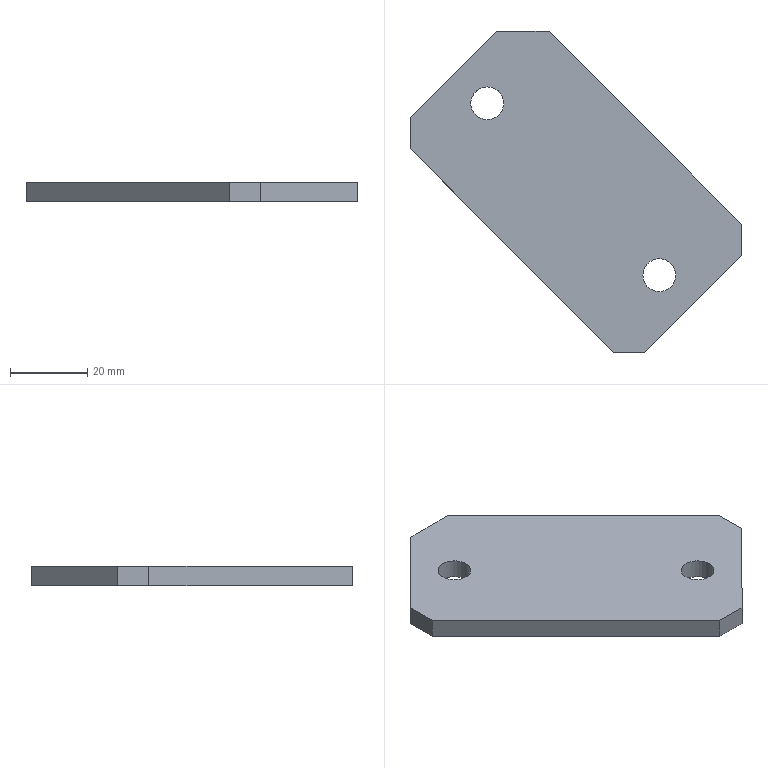Part | STEP file | gslz 2016.10.28-13_id546_x_t | 1 solid | 12 faces | box 85.974 x 83.146 x 5 mm | volume 19163 mm3 | plane 10 | cylinder 2 | commonest cylinder face diameters 8.5 x2
STEP:
#1=CARTESIAN_POINT('',(0.,0.,0.));
#2=DIRECTION('',(0.,0.,1.));
#3=DIRECTION('',(1.,0.,0.));
#4=AXIS2_PLACEMENT_3D('',#1,#2,#3);
#5=CARTESIAN_POINT('',(170.764,264.917,-94.));
#6=VERTEX_POINT('',#5);
#7=CARTESIAN_POINT('',(148.429,242.582,-94.));
#8=VERTEX_POINT('',#7);
#9=CARTESIAN_POINT('',(177.981,272.134,-94.));
#10=DIRECTION('',(-0.7071,-0.7071,0.));
#11=VECTOR('',#10,1.);
#12=LINE('',#9,#11);
#13=CARTESIAN_POINT('',(177.981,272.134,-99.));
#14=DIRECTION('',(-0.7071,0.7071,0.));
#15=DIRECTION('',(-0.7071,-0.7071,0.));
#16=AXIS2_PLACEMENT_3D('',#13,#14,#15);
#17=PLANE('',#16);
#18=CARTESIAN_POINT('',(0.,5.));
#19=DIRECTION('',(1.,0.));
#20=VECTOR('',#19,1.);
#21=LINE('',#18,#20);
#22=(GEOMETRIC_REPRESENTATION_CONTEXT(2)PARAMETRIC_REPRESENTATION_CONTEXT()REPRESENTATION_CONTEXT('',''));
#23=DEFINITIONAL_REPRESENTATION('',(#21),#22);
#24=PCURVE('',#17,#23);
#25=CARTESIAN_POINT('',(-1012.771,1462.886,-94.));
#26=DIRECTION('',(0.,0.,1.));
#27=DIRECTION('',(1.,0.,0.));
#28=AXIS2_PLACEMENT_3D('',#25,#26,#27);
#29=PLANE('',#28);
#30=CARTESIAN_POINT('',(1190.752,-1190.752));
#31=DIRECTION('',(-0.7071,-0.7071));
#32=VECTOR('',#31,1.);
#33=LINE('',#30,#32);
#34=(GEOMETRIC_REPRESENTATION_CONTEXT(2)PARAMETRIC_REPRESENTATION_CONTEXT()REPRESENTATION_CONTEXT('',''));
#35=DEFINITIONAL_REPRESENTATION('',(#33),#34);
#36=PCURVE('',#29,#35);
#37=SURFACE_CURVE('',#12,(#24,#36),.PCURVE_S1.);
#38=EDGE_CURVE('',#6,#8,#37,.T.);
#39=ORIENTED_EDGE('',*,*,#38,.F.);
#40=CARTESIAN_POINT('',(170.764,264.917,-99.));
#41=VERTEX_POINT('',#40);
#42=CARTESIAN_POINT('',(170.764,264.917,-99.));
#43=DIRECTION('',(0.,0.,1.));
#44=VECTOR('',#43,1.);
#45=LINE('',#42,#44);
#46=CARTESIAN_POINT('',(10.207,0.));
#47=DIRECTION('',(0.,1.));
#48=VECTOR('',#47,1.);
#49=LINE('',#46,#48);
#50=(GEOMETRIC_REPRESENTATION_CONTEXT(2)PARAMETRIC_REPRESENTATION_CONTEXT()REPRESENTATION_CONTEXT('',''));
#51=DEFINITIONAL_REPRESENTATION('',(#49),#50);
#52=PCURVE('',#17,#51);
#53=CARTESIAN_POINT('',(184.699,264.917,-99.));
#54=DIRECTION('',(0.,-1.,0.));
#55=DIRECTION('',(1.,0.,0.));
#56=AXIS2_PLACEMENT_3D('',#53,#54,#55);
#57=PLANE('',#56);
#58=CARTESIAN_POINT('',(-13.935,0.));
#59=DIRECTION('',(0.,1.));
#60=VECTOR('',#59,1.);
#61=LINE('',#58,#60);
#62=(GEOMETRIC_REPRESENTATION_CONTEXT(2)PARAMETRIC_REPRESENTATION_CONTEXT()REPRESENTATION_CONTEXT('',''));
#63=DEFINITIONAL_REPRESENTATION('',(#61),#62);
#64=PCURVE('',#57,#63);
#65=SURFACE_CURVE('',#45,(#52,#64),.PCURVE_S1.);
#66=EDGE_CURVE('',#41,#6,#65,.T.);
#67=ORIENTED_EDGE('',*,*,#66,.F.);
#68=CARTESIAN_POINT('',(148.429,242.582,-99.));
#69=VERTEX_POINT('',#68);
#70=CARTESIAN_POINT('',(177.981,272.134,-99.));
#71=DIRECTION('',(-0.7071,-0.7071,0.));
#72=VECTOR('',#71,1.);
#73=LINE('',#70,#72);
#74=CARTESIAN_POINT('',(0.,0.));
#75=DIRECTION('',(1.,0.));
#76=VECTOR('',#75,1.);
#77=LINE('',#74,#76);
#78=(GEOMETRIC_REPRESENTATION_CONTEXT(2)PARAMETRIC_REPRESENTATION_CONTEXT()REPRESENTATION_CONTEXT('',''));
#79=DEFINITIONAL_REPRESENTATION('',(#77),#78);
#80=PCURVE('',#17,#79);
#81=CARTESIAN_POINT('',(-1012.771,1462.886,-99.));
#82=DIRECTION('',(0.,0.,1.));
#83=DIRECTION('',(1.,0.,0.));
#84=AXIS2_PLACEMENT_3D('',#81,#82,#83);
#85=PLANE('',#84);
#86=CARTESIAN_POINT('',(1190.752,-1190.752));
#87=DIRECTION('',(-0.7071,-0.7071));
#88=VECTOR('',#87,1.);
#89=LINE('',#86,#88);
#90=(GEOMETRIC_REPRESENTATION_CONTEXT(2)PARAMETRIC_REPRESENTATION_CONTEXT()REPRESENTATION_CONTEXT('',''));
#91=DEFINITIONAL_REPRESENTATION('',(#89),#90);
#92=PCURVE('',#85,#91);
#93=SURFACE_CURVE('',#73,(#80,#92),.PCURVE_S1.);
#94=EDGE_CURVE('',#41,#69,#93,.T.);
#95=ORIENTED_EDGE('',*,*,#94,.T.);
#96=CARTESIAN_POINT('',(148.429,242.582,-99.));
#97=DIRECTION('',(0.,0.,1.));
#98=VECTOR('',#97,1.);
#99=LINE('',#96,#98);
#100=CARTESIAN_POINT('',(41.793,0.));
#101=DIRECTION('',(0.,1.));
#102=VECTOR('',#101,1.);
#103=LINE('',#100,#102);
#104=(GEOMETRIC_REPRESENTATION_CONTEXT(2)PARAMETRIC_REPRESENTATION_CONTEXT()REPRESENTATION_CONTEXT('',''));
#105=DEFINITIONAL_REPRESENTATION('',(#103),#104);
#106=PCURVE('',#17,#105);
#107=CARTESIAN_POINT('',(148.429,242.789,-99.));
#108=DIRECTION('',(1.,0.,0.));
#109=DIRECTION('',(0.,1.,0.));
#110=AXIS2_PLACEMENT_3D('',#107,#108,#109);
#111=PLANE('',#110);
#112=CARTESIAN_POINT('',(-0.2071,0.));
#113=DIRECTION('',(0.,1.));
#114=VECTOR('',#113,1.);
#115=LINE('',#112,#114);
#116=(GEOMETRIC_REPRESENTATION_CONTEXT(2)PARAMETRIC_REPRESENTATION_CONTEXT()REPRESENTATION_CONTEXT('',''));
#117=DEFINITIONAL_REPRESENTATION('',(#115),#116);
#118=PCURVE('',#111,#117);
#119=SURFACE_CURVE('',#99,(#106,#118),.PCURVE_S1.);
#120=EDGE_CURVE('',#69,#8,#119,.T.);
#121=ORIENTED_EDGE('',*,*,#120,.T.);
#122=EDGE_LOOP('',(#39,#67,#95,#121));
#123=FACE_BOUND('',#122,.T.);
#124=ADVANCED_FACE('',(#123),#17,.T.);
#125=CARTESIAN_POINT('',(184.492,264.917,-94.));
#126=VERTEX_POINT('',#125);
#127=CARTESIAN_POINT('',(-1012.771,264.917,-94.));
#128=DIRECTION('',(1.,0.,0.));
#129=VECTOR('',#128,1.);
#130=LINE('',#127,#129);
#131=CARTESIAN_POINT('',(-1197.469,5.));
#132=DIRECTION('',(1.,0.));
#133=VECTOR('',#132,1.);
#134=LINE('',#131,#133);
#135=(GEOMETRIC_REPRESENTATION_CONTEXT(2)PARAMETRIC_REPRESENTATION_CONTEXT()REPRESENTATION_CONTEXT('',''));
#136=DEFINITIONAL_REPRESENTATION('',(#134),#135);
#137=PCURVE('',#57,#136);
#138=CARTESIAN_POINT('',(0.,-1197.969));
#139=DIRECTION('',(1.,0.));
#140=VECTOR('',#139,1.);
#141=LINE('',#138,#140);
#142=(GEOMETRIC_REPRESENTATION_CONTEXT(2)PARAMETRIC_REPRESENTATION_CONTEXT()REPRESENTATION_CONTEXT('',''));
#143=DEFINITIONAL_REPRESENTATION('',(#141),#142);
#144=PCURVE('',#29,#143);
#145=SURFACE_CURVE('',#130,(#137,#144),.PCURVE_S1.);
#146=EDGE_CURVE('',#6,#126,#145,.T.);
#147=ORIENTED_EDGE('',*,*,#146,.T.);
#148=CARTESIAN_POINT('',(184.492,264.917,-99.));
#149=VERTEX_POINT('',#148);
#150=CARTESIAN_POINT('',(184.492,264.917,-99.));
#151=DIRECTION('',(0.,0.,1.));
#152=VECTOR('',#151,1.);
#153=LINE('',#150,#152);
#154=CARTESIAN_POINT('',(-0.2071,0.));
#155=DIRECTION('',(0.,1.));
#156=VECTOR('',#155,1.);
#157=LINE('',#154,#156);
#158=(GEOMETRIC_REPRESENTATION_CONTEXT(2)PARAMETRIC_REPRESENTATION_CONTEXT()REPRESENTATION_CONTEXT('',''));
#159=DEFINITIONAL_REPRESENTATION('',(#157),#158);
#160=PCURVE('',#57,#159);
#161=CARTESIAN_POINT('',(-1013.124,1462.533,-99.));
#162=DIRECTION('',(0.7071,0.7071,0.));
#163=DIRECTION('',(-0.7071,0.7071,0.));
#164=AXIS2_PLACEMENT_3D('',#161,#162,#163);
#165=PLANE('',#164);
#166=CARTESIAN_POINT('',(-1693.685,0.));
#167=DIRECTION('',(0.,1.));
#168=VECTOR('',#167,1.);
#169=LINE('',#166,#168);
#170=(GEOMETRIC_REPRESENTATION_CONTEXT(2)PARAMETRIC_REPRESENTATION_CONTEXT()REPRESENTATION_CONTEXT('',''));
#171=DEFINITIONAL_REPRESENTATION('',(#169),#170);
#172=PCURVE('',#165,#171);
#173=SURFACE_CURVE('',#153,(#160,#172),.PCURVE_S1.);
#174=EDGE_CURVE('',#149,#126,#173,.T.);
#175=ORIENTED_EDGE('',*,*,#174,.F.);
#176=CARTESIAN_POINT('',(-1012.771,264.917,-99.));
#177=DIRECTION('',(1.,0.,0.));
#178=VECTOR('',#177,1.);
#179=LINE('',#176,#178);
#180=CARTESIAN_POINT('',(-1197.469,0.));
#181=DIRECTION('',(1.,0.));
#182=VECTOR('',#181,1.);
#183=LINE('',#180,#182);
#184=(GEOMETRIC_REPRESENTATION_CONTEXT(2)PARAMETRIC_REPRESENTATION_CONTEXT()REPRESENTATION_CONTEXT('',''));
#185=DEFINITIONAL_REPRESENTATION('',(#183),#184);
#186=PCURVE('',#57,#185);
#187=CARTESIAN_POINT('',(0.,-1197.969));
#188=DIRECTION('',(1.,0.));
#189=VECTOR('',#188,1.);
#190=LINE('',#187,#189);
#191=(GEOMETRIC_REPRESENTATION_CONTEXT(2)PARAMETRIC_REPRESENTATION_CONTEXT()REPRESENTATION_CONTEXT('',''));
#192=DEFINITIONAL_REPRESENTATION('',(#190),#191);
#193=PCURVE('',#85,#192);
#194=SURFACE_CURVE('',#179,(#186,#193),.PCURVE_S1.);
#195=EDGE_CURVE('',#41,#149,#194,.T.);
#196=ORIENTED_EDGE('',*,*,#195,.F.);
#197=ORIENTED_EDGE('',*,*,#66,.T.);
#198=EDGE_LOOP('',(#147,#175,#196,#197));
#199=FACE_BOUND('',#198,.T.);
#200=ADVANCED_FACE('',(#199),#57,.F.);
#201=CARTESIAN_POINT('',(234.403,215.005,-94.));
#202=VERTEX_POINT('',#201);
#203=CARTESIAN_POINT('',(-1013.124,1462.533,-94.));
#204=DIRECTION('',(-0.7071,0.7071,0.));
#205=VECTOR('',#204,1.);
#206=LINE('',#203,#205);
#207=CARTESIAN_POINT('',(0.,5.));
#208=DIRECTION('',(1.,0.));
#209=VECTOR('',#208,1.);
#210=LINE('',#207,#209);
#211=(GEOMETRIC_REPRESENTATION_CONTEXT(2)PARAMETRIC_REPRESENTATION_CONTEXT()REPRESENTATION_CONTEXT('',''));
#212=DEFINITIONAL_REPRESENTATION('',(#210),#211);
#213=PCURVE('',#165,#212);
#214=CARTESIAN_POINT('',(-0.3536,-0.3536));
#215=DIRECTION('',(-0.7071,0.7071));
#216=VECTOR('',#215,1.);
#217=LINE('',#214,#216);
#218=(GEOMETRIC_REPRESENTATION_CONTEXT(2)PARAMETRIC_REPRESENTATION_CONTEXT()REPRESENTATION_CONTEXT('',''));
#219=DEFINITIONAL_REPRESENTATION('',(#217),#218);
#220=PCURVE('',#29,#219);
#221=SURFACE_CURVE('',#206,(#213,#220),.PCURVE_S1.);
#222=EDGE_CURVE('',#202,#126,#221,.T.);
#223=ORIENTED_EDGE('',*,*,#222,.F.);
#224=CARTESIAN_POINT('',(234.403,215.005,-99.));
#225=VERTEX_POINT('',#224);
#226=CARTESIAN_POINT('',(234.403,215.005,-99.));
#227=DIRECTION('',(0.,0.,1.));
#228=VECTOR('',#227,1.);
#229=LINE('',#226,#228);
#230=CARTESIAN_POINT('',(-1764.27,0.));
#231=DIRECTION('',(0.,1.));
#232=VECTOR('',#231,1.);
#233=LINE('',#230,#232);
#234=(GEOMETRIC_REPRESENTATION_CONTEXT(2)PARAMETRIC_REPRESENTATION_CONTEXT()REPRESENTATION_CONTEXT('',''));
#235=DEFINITIONAL_REPRESENTATION('',(#233),#234);
#236=PCURVE('',#165,#235);
#237=CARTESIAN_POINT('',(234.403,206.727,-99.));
#238=DIRECTION('',(-1.,0.,0.));
#239=DIRECTION('',(0.,-1.,0.));
#240=AXIS2_PLACEMENT_3D('',#237,#238,#239);
#241=PLANE('',#240);
#242=CARTESIAN_POINT('',(-8.278,0.));
#243=DIRECTION('',(0.,1.));
#244=VECTOR('',#243,1.);
#245=LINE('',#242,#244);
#246=(GEOMETRIC_REPRESENTATION_CONTEXT(2)PARAMETRIC_REPRESENTATION_CONTEXT()REPRESENTATION_CONTEXT('',''));
#247=DEFINITIONAL_REPRESENTATION('',(#245),#246);
#248=PCURVE('',#241,#247);
#249=SURFACE_CURVE('',#229,(#236,#248),.PCURVE_S1.);
#250=EDGE_CURVE('',#225,#202,#249,.T.);
#251=ORIENTED_EDGE('',*,*,#250,.F.);
#252=CARTESIAN_POINT('',(-1013.124,1462.533,-99.));
#253=DIRECTION('',(-0.7071,0.7071,0.));
#254=VECTOR('',#253,1.);
#255=LINE('',#252,#254);
#256=CARTESIAN_POINT('',(0.,0.));
#257=DIRECTION('',(1.,0.));
#258=VECTOR('',#257,1.);
#259=LINE('',#256,#258);
#260=(GEOMETRIC_REPRESENTATION_CONTEXT(2)PARAMETRIC_REPRESENTATION_CONTEXT()REPRESENTATION_CONTEXT('',''));
#261=DEFINITIONAL_REPRESENTATION('',(#259),#260);
#262=PCURVE('',#165,#261);
#263=CARTESIAN_POINT('',(-0.3536,-0.3536));
#264=DIRECTION('',(-0.7071,0.7071));
#265=VECTOR('',#264,1.);
#266=LINE('',#263,#265);
#267=(GEOMETRIC_REPRESENTATION_CONTEXT(2)PARAMETRIC_REPRESENTATION_CONTEXT()REPRESENTATION_CONTEXT('',''));
#268=DEFINITIONAL_REPRESENTATION('',(#266),#267);
#269=PCURVE('',#85,#268);
#270=SURFACE_CURVE('',#255,(#262,#269),.PCURVE_S1.);
#271=EDGE_CURVE('',#225,#149,#270,.T.);
#272=ORIENTED_EDGE('',*,*,#271,.T.);
#273=ORIENTED_EDGE('',*,*,#174,.T.);
#274=EDGE_LOOP('',(#223,#251,#272,#273));
#275=FACE_BOUND('',#274,.T.);
#276=ADVANCED_FACE('',(#275),#165,.T.);
#277=CARTESIAN_POINT('',(234.403,206.934,-94.));
#278=VERTEX_POINT('',#277);
#279=CARTESIAN_POINT('',(234.403,1462.886,-94.));
#280=DIRECTION('',(0.,-1.,0.));
#281=VECTOR('',#280,1.);
#282=LINE('',#279,#281);
#283=CARTESIAN_POINT('',(-1256.159,5.));
#284=DIRECTION('',(1.,0.));
#285=VECTOR('',#284,1.);
#286=LINE('',#283,#285);
#287=(GEOMETRIC_REPRESENTATION_CONTEXT(2)PARAMETRIC_REPRESENTATION_CONTEXT()REPRESENTATION_CONTEXT('',''));
#288=DEFINITIONAL_REPRESENTATION('',(#286),#287);
#289=PCURVE('',#241,#288);
#290=CARTESIAN_POINT('',(1247.174,0.));
#291=DIRECTION('',(0.,-1.));
#292=VECTOR('',#291,1.);
#293=LINE('',#290,#292);
#294=(GEOMETRIC_REPRESENTATION_CONTEXT(2)PARAMETRIC_REPRESENTATION_CONTEXT()REPRESENTATION_CONTEXT('',''));
#295=DEFINITIONAL_REPRESENTATION('',(#293),#294);
#296=PCURVE('',#29,#295);
#297=SURFACE_CURVE('',#282,(#289,#296),.PCURVE_S1.);
#298=EDGE_CURVE('',#202,#278,#297,.T.);
#299=ORIENTED_EDGE('',*,*,#298,.T.);
#300=CARTESIAN_POINT('',(234.403,206.934,-99.));
#301=VERTEX_POINT('',#300);
#302=CARTESIAN_POINT('',(234.403,206.934,-99.));
#303=DIRECTION('',(0.,0.,1.));
#304=VECTOR('',#303,1.);
#305=LINE('',#302,#304);
#306=CARTESIAN_POINT('',(-0.2071,0.));
#307=DIRECTION('',(0.,1.));
#308=VECTOR('',#307,1.);
#309=LINE('',#306,#308);
#310=(GEOMETRIC_REPRESENTATION_CONTEXT(2)PARAMETRIC_REPRESENTATION_CONTEXT()REPRESENTATION_CONTEXT('',''));
#311=DEFINITIONAL_REPRESENTATION('',(#309),#310);
#312=PCURVE('',#241,#311);
#313=CARTESIAN_POINT('',(238.793,211.323,-99.));
#314=DIRECTION('',(-0.7071,0.7071,0.));
#315=DIRECTION('',(-0.7071,-0.7071,0.));
#316=AXIS2_PLACEMENT_3D('',#313,#314,#315);
#317=PLANE('',#316);
#318=CARTESIAN_POINT('',(6.207,0.));
#319=DIRECTION('',(0.,1.));
#320=VECTOR('',#319,1.);
#321=LINE('',#318,#320);
#322=(GEOMETRIC_REPRESENTATION_CONTEXT(2)PARAMETRIC_REPRESENTATION_CONTEXT()REPRESENTATION_CONTEXT('',''));
#323=DEFINITIONAL_REPRESENTATION('',(#321),#322);
#324=PCURVE('',#317,#323);
#325=SURFACE_CURVE('',#305,(#312,#324),.PCURVE_S1.);
#326=EDGE_CURVE('',#301,#278,#325,.T.);
#327=ORIENTED_EDGE('',*,*,#326,.F.);
#328=CARTESIAN_POINT('',(234.403,1462.886,-99.));
#329=DIRECTION('',(0.,-1.,0.));
#330=VECTOR('',#329,1.);
#331=LINE('',#328,#330);
#332=CARTESIAN_POINT('',(-1256.159,0.));
#333=DIRECTION('',(1.,0.));
#334=VECTOR('',#333,1.);
#335=LINE('',#332,#334);
#336=(GEOMETRIC_REPRESENTATION_CONTEXT(2)PARAMETRIC_REPRESENTATION_CONTEXT()REPRESENTATION_CONTEXT('',''));
#337=DEFINITIONAL_REPRESENTATION('',(#335),#336);
#338=PCURVE('',#241,#337);
#339=CARTESIAN_POINT('',(1247.174,0.));
#340=DIRECTION('',(0.,-1.));
#341=VECTOR('',#340,1.);
#342=LINE('',#339,#341);
#343=(GEOMETRIC_REPRESENTATION_CONTEXT(2)PARAMETRIC_REPRESENTATION_CONTEXT()REPRESENTATION_CONTEXT('',''));
#344=DEFINITIONAL_REPRESENTATION('',(#342),#343);
#345=PCURVE('',#85,#344);
#346=SURFACE_CURVE('',#331,(#338,#345),.PCURVE_S1.);
#347=EDGE_CURVE('',#225,#301,#346,.T.);
#348=ORIENTED_EDGE('',*,*,#347,.F.);
#349=ORIENTED_EDGE('',*,*,#250,.T.);
#350=EDGE_LOOP('',(#299,#327,#348,#349));
#351=FACE_BOUND('',#350,.T.);
#352=ADVANCED_FACE('',(#351),#241,.F.);
#353=CARTESIAN_POINT('',(209.241,181.771,-94.));
#354=VERTEX_POINT('',#353);
#355=CARTESIAN_POINT('',(238.793,211.323,-94.));
#356=DIRECTION('',(-0.7071,-0.7071,0.));
#357=VECTOR('',#356,1.);
#358=LINE('',#355,#357);
#359=CARTESIAN_POINT('',(0.,5.));
#360=DIRECTION('',(1.,0.));
#361=VECTOR('',#360,1.);
#362=LINE('',#359,#361);
#363=(GEOMETRIC_REPRESENTATION_CONTEXT(2)PARAMETRIC_REPRESENTATION_CONTEXT()REPRESENTATION_CONTEXT('',''));
#364=DEFINITIONAL_REPRESENTATION('',(#362),#363);
#365=PCURVE('',#317,#364);
#366=CARTESIAN_POINT('',(1251.563,-1251.563));
#367=DIRECTION('',(-0.7071,-0.7071));
#368=VECTOR('',#367,1.);
#369=LINE('',#366,#368);
#370=(GEOMETRIC_REPRESENTATION_CONTEXT(2)PARAMETRIC_REPRESENTATION_CONTEXT()REPRESENTATION_CONTEXT('',''));
#371=DEFINITIONAL_REPRESENTATION('',(#369),#370);
#372=PCURVE('',#29,#371);
#373=SURFACE_CURVE('',#358,(#365,#372),.PCURVE_S1.);
#374=EDGE_CURVE('',#278,#354,#373,.T.);
#375=ORIENTED_EDGE('',*,*,#374,.T.);
#376=CARTESIAN_POINT('',(209.241,181.771,-99.));
#377=VERTEX_POINT('',#376);
#378=CARTESIAN_POINT('',(209.241,181.771,-99.));
#379=DIRECTION('',(0.,0.,1.));
#380=VECTOR('',#379,1.);
#381=LINE('',#378,#380);
#382=CARTESIAN_POINT('',(41.793,0.));
#383=DIRECTION('',(0.,1.));
#384=VECTOR('',#383,1.);
#385=LINE('',#382,#384);
#386=(GEOMETRIC_REPRESENTATION_CONTEXT(2)PARAMETRIC_REPRESENTATION_CONTEXT()REPRESENTATION_CONTEXT('',''));
#387=DEFINITIONAL_REPRESENTATION('',(#385),#386);
#388=PCURVE('',#317,#387);
#389=CARTESIAN_POINT('',(200.962,181.771,-99.));
#390=DIRECTION('',(0.,1.,0.));
#391=DIRECTION('',(-1.,0.,0.));
#392=AXIS2_PLACEMENT_3D('',#389,#390,#391);
#393=PLANE('',#392);
#394=CARTESIAN_POINT('',(-8.278,0.));
#395=DIRECTION('',(0.,1.));
#396=VECTOR('',#395,1.);
#397=LINE('',#394,#396);
#398=(GEOMETRIC_REPRESENTATION_CONTEXT(2)PARAMETRIC_REPRESENTATION_CONTEXT()REPRESENTATION_CONTEXT('',''));
#399=DEFINITIONAL_REPRESENTATION('',(#397),#398);
#400=PCURVE('',#393,#399);
#401=SURFACE_CURVE('',#381,(#388,#400),.PCURVE_S1.);
#402=EDGE_CURVE('',#377,#354,#401,.T.);
#403=ORIENTED_EDGE('',*,*,#402,.F.);
#404=CARTESIAN_POINT('',(238.793,211.323,-99.));
#405=DIRECTION('',(-0.7071,-0.7071,0.));
#406=VECTOR('',#405,1.);
#407=LINE('',#404,#406);
#408=CARTESIAN_POINT('',(0.,0.));
#409=DIRECTION('',(1.,0.));
#410=VECTOR('',#409,1.);
#411=LINE('',#408,#410);
#412=(GEOMETRIC_REPRESENTATION_CONTEXT(2)PARAMETRIC_REPRESENTATION_CONTEXT()REPRESENTATION_CONTEXT('',''));
#413=DEFINITIONAL_REPRESENTATION('',(#411),#412);
#414=PCURVE('',#317,#413);
#415=CARTESIAN_POINT('',(1251.563,-1251.563));
#416=DIRECTION('',(-0.7071,-0.7071));
#417=VECTOR('',#416,1.);
#418=LINE('',#415,#417);
#419=(GEOMETRIC_REPRESENTATION_CONTEXT(2)PARAMETRIC_REPRESENTATION_CONTEXT()REPRESENTATION_CONTEXT('',''));
#420=DEFINITIONAL_REPRESENTATION('',(#418),#419);
#421=PCURVE('',#85,#420);
#422=SURFACE_CURVE('',#407,(#414,#421),.PCURVE_S1.);
#423=EDGE_CURVE('',#301,#377,#422,.T.);
#424=ORIENTED_EDGE('',*,*,#423,.F.);
#425=ORIENTED_EDGE('',*,*,#326,.T.);
#426=EDGE_LOOP('',(#375,#403,#424,#425));
#427=FACE_BOUND('',#426,.T.);
#428=ADVANCED_FACE('',(#427),#317,.F.);
#429=CARTESIAN_POINT('',(201.169,181.771,-94.));
#430=VERTEX_POINT('',#429);
#431=CARTESIAN_POINT('',(-1012.771,181.771,-94.));
#432=DIRECTION('',(-1.,0.,0.));
#433=VECTOR('',#432,1.);
#434=LINE('',#431,#433);
#435=CARTESIAN_POINT('',(1213.733,5.));
#436=DIRECTION('',(1.,0.));
#437=VECTOR('',#436,1.);
#438=LINE('',#435,#437);
#439=(GEOMETRIC_REPRESENTATION_CONTEXT(2)PARAMETRIC_REPRESENTATION_CONTEXT()REPRESENTATION_CONTEXT('',''));
#440=DEFINITIONAL_REPRESENTATION('',(#438),#439);
#441=PCURVE('',#393,#440);
#442=CARTESIAN_POINT('',(0.,-1281.115));
#443=DIRECTION('',(-1.,0.));
#444=VECTOR('',#443,1.);
#445=LINE('',#442,#444);
#446=(GEOMETRIC_REPRESENTATION_CONTEXT(2)PARAMETRIC_REPRESENTATION_CONTEXT()REPRESENTATION_CONTEXT('',''));
#447=DEFINITIONAL_REPRESENTATION('',(#445),#446);
#448=PCURVE('',#29,#447);
#449=SURFACE_CURVE('',#434,(#441,#448),.PCURVE_S1.);
#450=EDGE_CURVE('',#354,#430,#449,.T.);
#451=ORIENTED_EDGE('',*,*,#450,.T.);
#452=CARTESIAN_POINT('',(201.169,181.771,-99.));
#453=VERTEX_POINT('',#452);
#454=CARTESIAN_POINT('',(201.169,181.771,-99.));
#455=DIRECTION('',(0.,0.,1.));
#456=VECTOR('',#455,1.);
#457=LINE('',#454,#456);
#458=CARTESIAN_POINT('',(-0.2071,0.));
#459=DIRECTION('',(0.,1.));
#460=VECTOR('',#459,1.);
#461=LINE('',#458,#460);
#462=(GEOMETRIC_REPRESENTATION_CONTEXT(2)PARAMETRIC_REPRESENTATION_CONTEXT()REPRESENTATION_CONTEXT('',''));
#463=DEFINITIONAL_REPRESENTATION('',(#461),#462);
#464=PCURVE('',#393,#463);
#465=CARTESIAN_POINT('',(-1046.358,1429.299,-99.));
#466=DIRECTION('',(0.7071,0.7071,0.));
#467=DIRECTION('',(-0.7071,0.7071,0.));
#468=AXIS2_PLACEMENT_3D('',#465,#466,#467);
#469=PLANE('',#468);
#470=CARTESIAN_POINT('',(-1764.27,0.));
#471=DIRECTION('',(0.,1.));
#472=VECTOR('',#471,1.);
#473=LINE('',#470,#472);
#474=(GEOMETRIC_REPRESENTATION_CONTEXT(2)PARAMETRIC_REPRESENTATION_CONTEXT()REPRESENTATION_CONTEXT('',''));
#475=DEFINITIONAL_REPRESENTATION('',(#473),#474);
#476=PCURVE('',#469,#475);
#477=SURFACE_CURVE('',#457,(#464,#476),.PCURVE_S1.);
#478=EDGE_CURVE('',#453,#430,#477,.T.);
#479=ORIENTED_EDGE('',*,*,#478,.F.);
#480=CARTESIAN_POINT('',(-1012.771,181.771,-99.));
#481=DIRECTION('',(-1.,0.,0.));
#482=VECTOR('',#481,1.);
#483=LINE('',#480,#482);
#484=CARTESIAN_POINT('',(1213.733,0.));
#485=DIRECTION('',(1.,0.));
#486=VECTOR('',#485,1.);
#487=LINE('',#484,#486);
#488=(GEOMETRIC_REPRESENTATION_CONTEXT(2)PARAMETRIC_REPRESENTATION_CONTEXT()REPRESENTATION_CONTEXT('',''));
#489=DEFINITIONAL_REPRESENTATION('',(#487),#488);
#490=PCURVE('',#393,#489);
#491=CARTESIAN_POINT('',(0.,-1281.115));
#492=DIRECTION('',(-1.,0.));
#493=VECTOR('',#492,1.);
#494=LINE('',#491,#493);
#495=(GEOMETRIC_REPRESENTATION_CONTEXT(2)PARAMETRIC_REPRESENTATION_CONTEXT()REPRESENTATION_CONTEXT('',''));
#496=DEFINITIONAL_REPRESENTATION('',(#494),#495);
#497=PCURVE('',#85,#496);
#498=SURFACE_CURVE('',#483,(#490,#497),.PCURVE_S1.);
#499=EDGE_CURVE('',#377,#453,#498,.T.);
#500=ORIENTED_EDGE('',*,*,#499,.F.);
#501=ORIENTED_EDGE('',*,*,#402,.T.);
#502=EDGE_LOOP('',(#451,#479,#500,#501));
#503=FACE_BOUND('',#502,.T.);
#504=ADVANCED_FACE('',(#503),#393,.F.);
#505=CARTESIAN_POINT('',(148.429,234.511,-94.));
#506=VERTEX_POINT('',#505);
#507=CARTESIAN_POINT('',(-1046.358,1429.299,-94.));
#508=DIRECTION('',(-0.7071,0.7071,0.));
#509=VECTOR('',#508,1.);
#510=LINE('',#507,#509);
#511=CARTESIAN_POINT('',(0.,5.));
#512=DIRECTION('',(1.,0.));
#513=VECTOR('',#512,1.);
#514=LINE('',#511,#513);
#515=(GEOMETRIC_REPRESENTATION_CONTEXT(2)PARAMETRIC_REPRESENTATION_CONTEXT()REPRESENTATION_CONTEXT('',''));
#516=DEFINITIONAL_REPRESENTATION('',(#514),#515);
#517=PCURVE('',#469,#516);
#518=CARTESIAN_POINT('',(-33.588,-33.588));
#519=DIRECTION('',(-0.7071,0.7071));
#520=VECTOR('',#519,1.);
#521=LINE('',#518,#520);
#522=(GEOMETRIC_REPRESENTATION_CONTEXT(2)PARAMETRIC_REPRESENTATION_CONTEXT()REPRESENTATION_CONTEXT('',''));
#523=DEFINITIONAL_REPRESENTATION('',(#521),#522);
#524=PCURVE('',#29,#523);
#525=SURFACE_CURVE('',#510,(#517,#524),.PCURVE_S1.);
#526=EDGE_CURVE('',#430,#506,#525,.T.);
#527=ORIENTED_EDGE('',*,*,#526,.T.);
#528=CARTESIAN_POINT('',(148.429,234.511,-99.));
#529=VERTEX_POINT('',#528);
#530=CARTESIAN_POINT('',(148.429,234.511,-99.));
#531=DIRECTION('',(0.,0.,1.));
#532=VECTOR('',#531,1.);
#533=LINE('',#530,#532);
#534=CARTESIAN_POINT('',(-1689.685,0.));
#535=DIRECTION('',(0.,1.));
#536=VECTOR('',#535,1.);
#537=LINE('',#534,#536);
#538=(GEOMETRIC_REPRESENTATION_CONTEXT(2)PARAMETRIC_REPRESENTATION_CONTEXT()REPRESENTATION_CONTEXT('',''));
#539=DEFINITIONAL_REPRESENTATION('',(#537),#538);
#540=PCURVE('',#469,#539);
#541=CARTESIAN_POINT('',(-8.278,0.));
#542=DIRECTION('',(0.,1.));
#543=VECTOR('',#542,1.);
#544=LINE('',#541,#543);
#545=(GEOMETRIC_REPRESENTATION_CONTEXT(2)PARAMETRIC_REPRESENTATION_CONTEXT()REPRESENTATION_CONTEXT('',''));
#546=DEFINITIONAL_REPRESENTATION('',(#544),#545);
#547=PCURVE('',#111,#546);
#548=SURFACE_CURVE('',#533,(#540,#547),.PCURVE_S1.);
#549=EDGE_CURVE('',#529,#506,#548,.T.);
#550=ORIENTED_EDGE('',*,*,#549,.F.);
#551=CARTESIAN_POINT('',(-1046.358,1429.299,-99.));
#552=DIRECTION('',(-0.7071,0.7071,0.));
#553=VECTOR('',#552,1.);
#554=LINE('',#551,#553);
#555=CARTESIAN_POINT('',(0.,0.));
#556=DIRECTION('',(1.,0.));
#557=VECTOR('',#556,1.);
#558=LINE('',#555,#557);
#559=(GEOMETRIC_REPRESENTATION_CONTEXT(2)PARAMETRIC_REPRESENTATION_CONTEXT()REPRESENTATION_CONTEXT('',''));
#560=DEFINITIONAL_REPRESENTATION('',(#558),#559);
#561=PCURVE('',#469,#560);
#562=CARTESIAN_POINT('',(-33.588,-33.588));
#563=DIRECTION('',(-0.7071,0.7071));
#564=VECTOR('',#563,1.);
#565=LINE('',#562,#564);
#566=(GEOMETRIC_REPRESENTATION_CONTEXT(2)PARAMETRIC_REPRESENTATION_CONTEXT()REPRESENTATION_CONTEXT('',''));
#567=DEFINITIONAL_REPRESENTATION('',(#565),#566);
#568=PCURVE('',#85,#567);
#569=SURFACE_CURVE('',#554,(#561,#568),.PCURVE_S1.);
#570=EDGE_CURVE('',#453,#529,#569,.T.);
#571=ORIENTED_EDGE('',*,*,#570,.F.);
#572=ORIENTED_EDGE('',*,*,#478,.T.);
#573=EDGE_LOOP('',(#527,#550,#571,#572));
#574=FACE_BOUND('',#573,.T.);
#575=ADVANCED_FACE('',(#574),#469,.F.);
#576=CARTESIAN_POINT('',(168.435,242.075,-99.));
#577=VERTEX_POINT('',#576);
#578=CARTESIAN_POINT('',(168.435,246.325,-99.));
#579=DIRECTION('',(0.,0.,1.));
#580=DIRECTION('',(0.,-1.,0.));
#581=AXIS2_PLACEMENT_3D('',#578,#579,#580);
#582=CIRCLE('',#581,4.25);
#583=CARTESIAN_POINT('',(168.435,246.325,-99.));
#584=DIRECTION('',(0.,0.,1.));
#585=DIRECTION('',(1.,0.,0.));
#586=AXIS2_PLACEMENT_3D('',#583,#584,#585);
#587=CYLINDRICAL_SURFACE('',#586,4.25);
#588=CARTESIAN_POINT('',(4.712,0.));
#589=DIRECTION('',(1.,0.));
#590=VECTOR('',#589,1.);
#591=LINE('',#588,#590);
#592=(GEOMETRIC_REPRESENTATION_CONTEXT(2)PARAMETRIC_REPRESENTATION_CONTEXT()REPRESENTATION_CONTEXT('',''));
#593=DEFINITIONAL_REPRESENTATION('',(#591),#592);
#594=PCURVE('',#587,#593);
#595=CARTESIAN_POINT('',(1181.206,-1216.561));
#596=DIRECTION('',(0.,-1.));
#597=AXIS2_PLACEMENT_2D('',#595,#596);
#598=CIRCLE('',#597,4.25);
#599=(GEOMETRIC_REPRESENTATION_CONTEXT(2)PARAMETRIC_REPRESENTATION_CONTEXT()REPRESENTATION_CONTEXT('',''));
#600=DEFINITIONAL_REPRESENTATION('',(#598),#599);
#601=PCURVE('',#85,#600);
#602=SURFACE_CURVE('',#582,(#594,#601),.PCURVE_S1.);
#603=EDGE_CURVE('',#577,#577,#602,.T.);
#604=ORIENTED_EDGE('',*,*,#603,.T.);
#605=CARTESIAN_POINT('',(168.435,242.075,-94.));
#606=VERTEX_POINT('',#605);
#607=CARTESIAN_POINT('',(168.435,242.075,-99.));
#608=CARTESIAN_POINT('',(168.435,242.075,-94.));
#609=B_SPLINE_CURVE_WITH_KNOTS('',1,(#607,#608),.UNSPECIFIED.,.F.,.F.,(2,2),(0.,5.),.PIECEWISE_BEZIER_KNOTS.);
#610=CARTESIAN_POINT('',(10.996,0.));
#611=DIRECTION('',(0.,1.));
#612=VECTOR('',#611,1.);
#613=LINE('',#610,#612);
#614=(GEOMETRIC_REPRESENTATION_CONTEXT(2)PARAMETRIC_REPRESENTATION_CONTEXT()REPRESENTATION_CONTEXT('',''));
#615=DEFINITIONAL_REPRESENTATION('',(#613),#614);
#616=PCURVE('',#587,#615);
#617=CARTESIAN_POINT('',(4.712,0.));
#618=DIRECTION('',(0.,1.));
#619=VECTOR('',#618,1.);
#620=LINE('',#617,#619);
#621=(GEOMETRIC_REPRESENTATION_CONTEXT(2)PARAMETRIC_REPRESENTATION_CONTEXT()REPRESENTATION_CONTEXT('',''));
#622=DEFINITIONAL_REPRESENTATION('',(#620),#621);
#623=PCURVE('',#587,#622);
#624=SEAM_CURVE('',#609,(#616,#623),.PCURVE_S1.);
#625=EDGE_CURVE('',#577,#606,#624,.T.);
#626=ORIENTED_EDGE('',*,*,#625,.T.);
#627=CARTESIAN_POINT('',(168.435,246.325,-94.));
#628=DIRECTION('',(0.,0.,1.));
#629=DIRECTION('',(0.,-1.,0.));
#630=AXIS2_PLACEMENT_3D('',#627,#628,#629);
#631=CIRCLE('',#630,4.25);
#632=CARTESIAN_POINT('',(4.712,5.));
#633=DIRECTION('',(1.,0.));
#634=VECTOR('',#633,1.);
#635=LINE('',#632,#634);
#636=(GEOMETRIC_REPRESENTATION_CONTEXT(2)PARAMETRIC_REPRESENTATION_CONTEXT()REPRESENTATION_CONTEXT('',''));
#637=DEFINITIONAL_REPRESENTATION('',(#635),#636);
#638=PCURVE('',#587,#637);
#639=CARTESIAN_POINT('',(1181.206,-1216.561));
#640=DIRECTION('',(0.,-1.));
#641=AXIS2_PLACEMENT_2D('',#639,#640);
#642=CIRCLE('',#641,4.25);
#643=(GEOMETRIC_REPRESENTATION_CONTEXT(2)PARAMETRIC_REPRESENTATION_CONTEXT()REPRESENTATION_CONTEXT('',''));
#644=DEFINITIONAL_REPRESENTATION('',(#642),#643);
#645=PCURVE('',#29,#644);
#646=SURFACE_CURVE('',#631,(#638,#645),.PCURVE_S1.);
#647=EDGE_CURVE('',#606,#606,#646,.T.);
#648=ORIENTED_EDGE('',*,*,#647,.F.);
#649=ORIENTED_EDGE('',*,*,#625,.F.);
#650=EDGE_LOOP('',(#604,#626,#648,#649));
#651=FACE_BOUND('',#650,.F.);
#652=ADVANCED_FACE('',(#651),#587,.F.);
#653=CARTESIAN_POINT('',(148.429,1462.886,-94.));
#654=DIRECTION('',(0.,1.,0.));
#655=VECTOR('',#654,1.);
#656=LINE('',#653,#655);
#657=CARTESIAN_POINT('',(1220.097,5.));
#658=DIRECTION('',(1.,0.));
#659=VECTOR('',#658,1.);
#660=LINE('',#657,#659);
#661=(GEOMETRIC_REPRESENTATION_CONTEXT(2)PARAMETRIC_REPRESENTATION_CONTEXT()REPRESENTATION_CONTEXT('',''));
#662=DEFINITIONAL_REPRESENTATION('',(#660),#661);
#663=PCURVE('',#111,#662);
#664=CARTESIAN_POINT('',(1161.2,0.));
#665=DIRECTION('',(0.,1.));
#666=VECTOR('',#665,1.);
#667=LINE('',#664,#666);
#668=(GEOMETRIC_REPRESENTATION_CONTEXT(2)PARAMETRIC_REPRESENTATION_CONTEXT()REPRESENTATION_CONTEXT('',''));
#669=DEFINITIONAL_REPRESENTATION('',(#667),#668);
#670=PCURVE('',#29,#669);
#671=SURFACE_CURVE('',#656,(#663,#670),.PCURVE_S1.);
#672=EDGE_CURVE('',#506,#8,#671,.T.);
#673=ORIENTED_EDGE('',*,*,#672,.T.);
#674=ORIENTED_EDGE('',*,*,#120,.F.);
#675=CARTESIAN_POINT('',(148.429,1462.886,-99.));
#676=DIRECTION('',(0.,1.,0.));
#677=VECTOR('',#676,1.);
#678=LINE('',#675,#677);
#679=CARTESIAN_POINT('',(1220.097,0.));
#680=DIRECTION('',(1.,0.));
#681=VECTOR('',#680,1.);
#682=LINE('',#679,#681);
#683=(GEOMETRIC_REPRESENTATION_CONTEXT(2)PARAMETRIC_REPRESENTATION_CONTEXT()REPRESENTATION_CONTEXT('',''));
#684=DEFINITIONAL_REPRESENTATION('',(#682),#683);
#685=PCURVE('',#111,#684);
#686=CARTESIAN_POINT('',(1161.2,0.));
#687=DIRECTION('',(0.,1.));
#688=VECTOR('',#687,1.);
#689=LINE('',#686,#688);
#690=(GEOMETRIC_REPRESENTATION_CONTEXT(2)PARAMETRIC_REPRESENTATION_CONTEXT()REPRESENTATION_CONTEXT('',''));
#691=DEFINITIONAL_REPRESENTATION('',(#689),#690);
#692=PCURVE('',#85,#691);
#693=SURFACE_CURVE('',#678,(#685,#692),.PCURVE_S1.);
#694=EDGE_CURVE('',#529,#69,#693,.T.);
#695=ORIENTED_EDGE('',*,*,#694,.F.);
#696=ORIENTED_EDGE('',*,*,#549,.T.);
#697=EDGE_LOOP('',(#673,#674,#695,#696));
#698=FACE_BOUND('',#697,.T.);
#699=ADVANCED_FACE('',(#698),#111,.F.);
#700=CARTESIAN_POINT('',(208.733,201.777,-99.));
#701=VERTEX_POINT('',#700);
#702=CARTESIAN_POINT('',(212.983,201.777,-99.));
#703=DIRECTION('',(0.,0.,-1.));
#704=DIRECTION('',(-1.,0.,0.));
#705=AXIS2_PLACEMENT_3D('',#702,#703,#704);
#706=CIRCLE('',#705,4.25);
#707=CARTESIAN_POINT('',(212.983,201.777,-99.));
#708=DIRECTION('',(0.,0.,1.));
#709=DIRECTION('',(1.,0.,0.));
#710=AXIS2_PLACEMENT_3D('',#707,#708,#709);
#711=CYLINDRICAL_SURFACE('',#710,4.25);
#712=CARTESIAN_POINT('',(9.425,0.));
#713=DIRECTION('',(-1.,0.));
#714=VECTOR('',#713,1.);
#715=LINE('',#712,#714);
#716=(GEOMETRIC_REPRESENTATION_CONTEXT(2)PARAMETRIC_REPRESENTATION_CONTEXT()REPRESENTATION_CONTEXT('',''));
#717=DEFINITIONAL_REPRESENTATION('',(#715),#716);
#718=PCURVE('',#711,#717);
#719=CARTESIAN_POINT('',(1221.504,-1261.109));
#720=CARTESIAN_POINT('',(1221.504,-1253.748));
#721=CARTESIAN_POINT('',(1227.879,-1257.428));
#722=CARTESIAN_POINT('',(1234.254,-1261.109));
#723=CARTESIAN_POINT('',(1227.879,-1264.79));
#724=CARTESIAN_POINT('',(1221.504,-1268.47));
#725=CARTESIAN_POINT('',(1221.504,-1261.109));
#726=(BOUNDED_CURVE()B_SPLINE_CURVE(2,(#719,#720,#721,#722,#723,#724,#725),.UNSPECIFIED.,.T.,.F.)B_SPLINE_CURVE_WITH_KNOTS((1,2,2,2,2,1),(-2.094,0.,2.094,4.189,6.283,8.378),.UNSPECIFIED.)CURVE()GEOMETRIC_REPRESENTATION_ITEM()RATIONAL_B_SPLINE_CURVE((1.,0.5,1.,0.5,1.,0.5,1.))REPRESENTATION_ITEM(''));
#727=(GEOMETRIC_REPRESENTATION_CONTEXT(2)PARAMETRIC_REPRESENTATION_CONTEXT()REPRESENTATION_CONTEXT('',''));
#728=DEFINITIONAL_REPRESENTATION('',(#726),#727);
#729=PCURVE('',#85,#728);
#730=SURFACE_CURVE('',#706,(#718,#729),.PCURVE_S1.);
#731=EDGE_CURVE('',#701,#701,#730,.T.);
#732=ORIENTED_EDGE('',*,*,#731,.F.);
#733=CARTESIAN_POINT('',(208.733,201.777,-94.));
#734=VERTEX_POINT('',#733);
#735=CARTESIAN_POINT('',(208.733,201.777,-99.));
#736=CARTESIAN_POINT('',(208.733,201.777,-94.));
#737=B_SPLINE_CURVE_WITH_KNOTS('',1,(#735,#736),.UNSPECIFIED.,.F.,.F.,(2,2),(0.,5.),.PIECEWISE_BEZIER_KNOTS.);
#738=CARTESIAN_POINT('',(9.425,0.));
#739=DIRECTION('',(0.,1.));
#740=VECTOR('',#739,1.);
#741=LINE('',#738,#740);
#742=(GEOMETRIC_REPRESENTATION_CONTEXT(2)PARAMETRIC_REPRESENTATION_CONTEXT()REPRESENTATION_CONTEXT('',''));
#743=DEFINITIONAL_REPRESENTATION('',(#741),#742);
#744=PCURVE('',#711,#743);
#745=CARTESIAN_POINT('',(3.142,0.));
#746=DIRECTION('',(0.,1.));
#747=VECTOR('',#746,1.);
#748=LINE('',#745,#747);
#749=(GEOMETRIC_REPRESENTATION_CONTEXT(2)PARAMETRIC_REPRESENTATION_CONTEXT()REPRESENTATION_CONTEXT('',''));
#750=DEFINITIONAL_REPRESENTATION('',(#748),#749);
#751=PCURVE('',#711,#750);
#752=SEAM_CURVE('',#737,(#744,#751),.PCURVE_S1.);
#753=EDGE_CURVE('',#701,#734,#752,.T.);
#754=ORIENTED_EDGE('',*,*,#753,.T.);
#755=CARTESIAN_POINT('',(212.983,201.777,-94.));
#756=DIRECTION('',(0.,0.,-1.));
#757=DIRECTION('',(-1.,0.,0.));
#758=AXIS2_PLACEMENT_3D('',#755,#756,#757);
#759=CIRCLE('',#758,4.25);
#760=CARTESIAN_POINT('',(9.425,5.));
#761=DIRECTION('',(-1.,0.));
#762=VECTOR('',#761,1.);
#763=LINE('',#760,#762);
#764=(GEOMETRIC_REPRESENTATION_CONTEXT(2)PARAMETRIC_REPRESENTATION_CONTEXT()REPRESENTATION_CONTEXT('',''));
#765=DEFINITIONAL_REPRESENTATION('',(#763),#764);
#766=PCURVE('',#711,#765);
#767=CARTESIAN_POINT('',(1221.504,-1261.109));
#768=CARTESIAN_POINT('',(1221.504,-1253.748));
#769=CARTESIAN_POINT('',(1227.879,-1257.428));
#770=CARTESIAN_POINT('',(1234.254,-1261.109));
#771=CARTESIAN_POINT('',(1227.879,-1264.79));
#772=CARTESIAN_POINT('',(1221.504,-1268.47));
#773=CARTESIAN_POINT('',(1221.504,-1261.109));
#774=(BOUNDED_CURVE()B_SPLINE_CURVE(2,(#767,#768,#769,#770,#771,#772,#773),.UNSPECIFIED.,.T.,.F.)B_SPLINE_CURVE_WITH_KNOTS((1,2,2,2,2,1),(-2.094,0.,2.094,4.189,6.283,8.378),.UNSPECIFIED.)CURVE()GEOMETRIC_REPRESENTATION_ITEM()RATIONAL_B_SPLINE_CURVE((1.,0.5,1.,0.5,1.,0.5,1.))REPRESENTATION_ITEM(''));
#775=(GEOMETRIC_REPRESENTATION_CONTEXT(2)PARAMETRIC_REPRESENTATION_CONTEXT()REPRESENTATION_CONTEXT('',''));
#776=DEFINITIONAL_REPRESENTATION('',(#774),#775);
#777=PCURVE('',#29,#776);
#778=SURFACE_CURVE('',#759,(#766,#777),.PCURVE_S1.);
#779=EDGE_CURVE('',#734,#734,#778,.T.);
#780=ORIENTED_EDGE('',*,*,#779,.T.);
#781=ORIENTED_EDGE('',*,*,#753,.F.);
#782=EDGE_LOOP('',(#732,#754,#780,#781));
#783=FACE_BOUND('',#782,.F.);
#784=ADVANCED_FACE('',(#783),#711,.F.);
#785=ORIENTED_EDGE('',*,*,#94,.F.);
#786=ORIENTED_EDGE('',*,*,#195,.T.);
#787=ORIENTED_EDGE('',*,*,#271,.F.);
#788=ORIENTED_EDGE('',*,*,#347,.T.);
#789=ORIENTED_EDGE('',*,*,#423,.T.);
#790=ORIENTED_EDGE('',*,*,#499,.T.);
#791=ORIENTED_EDGE('',*,*,#570,.T.);
#792=ORIENTED_EDGE('',*,*,#694,.T.);
#793=EDGE_LOOP('',(#785,#786,#787,#788,#789,#790,#791,#792));
#794=FACE_BOUND('',#793,.T.);
#795=ORIENTED_EDGE('',*,*,#603,.T.);
#796=EDGE_LOOP('',(#795));
#797=FACE_BOUND('',#796,.T.);
#798=ORIENTED_EDGE('',*,*,#731,.F.);
#799=EDGE_LOOP('',(#798));
#800=FACE_BOUND('',#799,.T.);
#801=ADVANCED_FACE('',(#794,#797,#800),#85,.F.);
#802=ORIENTED_EDGE('',*,*,#38,.T.);
#803=ORIENTED_EDGE('',*,*,#672,.F.);
#804=ORIENTED_EDGE('',*,*,#526,.F.);
#805=ORIENTED_EDGE('',*,*,#450,.F.);
#806=ORIENTED_EDGE('',*,*,#374,.F.);
#807=ORIENTED_EDGE('',*,*,#298,.F.);
#808=ORIENTED_EDGE('',*,*,#222,.T.);
#809=ORIENTED_EDGE('',*,*,#146,.F.);
#810=EDGE_LOOP('',(#802,#803,#804,#805,#806,#807,#808,#809));
#811=FACE_BOUND('',#810,.T.);
#812=ORIENTED_EDGE('',*,*,#647,.F.);
#813=EDGE_LOOP('',(#812));
#814=FACE_BOUND('',#813,.T.);
#815=ORIENTED_EDGE('',*,*,#779,.T.);
#816=EDGE_LOOP('',(#815));
#817=FACE_BOUND('',#816,.T.);
#818=ADVANCED_FACE('',(#811,#814,#817),#29,.T.);
#819=CLOSED_SHELL('',(#124,#200,#276,#352,#428,#504,#575,#652,#699,#784,#801,#818));
#820=MANIFOLD_SOLID_BREP('',#819);
#821=(LENGTH_UNIT()NAMED_UNIT(*)SI_UNIT(.MILLI.,.METRE.));
#822=UNCERTAINTY_MEASURE_WITH_UNIT(LENGTH_MEASURE(0.000002),#821,'','');
#823=(NAMED_UNIT(*)PLANE_ANGLE_UNIT()SI_UNIT($,.RADIAN.));
#824=(NAMED_UNIT(*)SI_UNIT($,.STERADIAN.)SOLID_ANGLE_UNIT());
#825=(GEOMETRIC_REPRESENTATION_CONTEXT(3)GLOBAL_UNCERTAINTY_ASSIGNED_CONTEXT((#822))GLOBAL_UNIT_ASSIGNED_CONTEXT((#821,#823,#824))REPRESENTATION_CONTEXT('',''));
#826=ADVANCED_BREP_SHAPE_REPRESENTATION('',(#4,#820),#825);